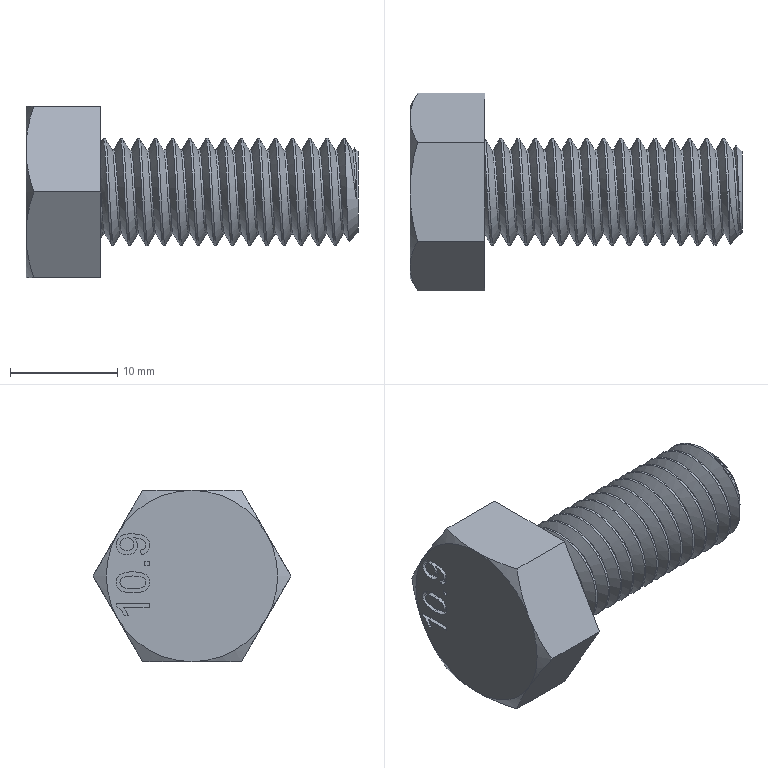Part | SolidWorks | features ICE 3, Chamfer 1, Extrusion 1, Helix 1, Revolution 1, Scale 1, SweepCut 1 | 1 solid | 91 faces | box 31 x 18.475 x 16 mm | volume 3064 mm3 | cylinder 30 | spline 28 | plane 25 | cone 8 | commonest cylinder face diameters 10 x30